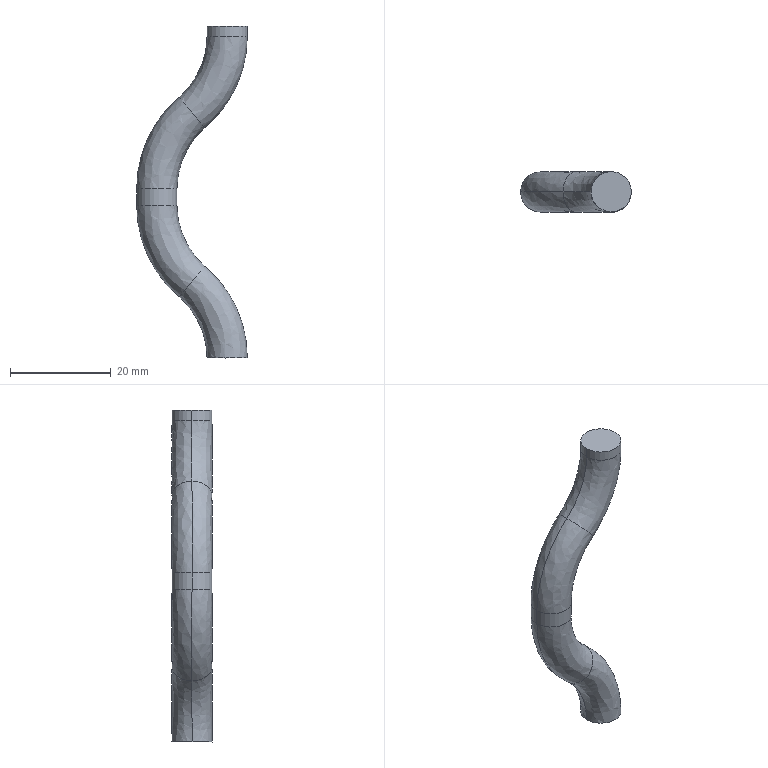Part | SolidWorks | features BaseBody 1 | 1 solid | 14 faces | box 22 x 8 x 66 mm | volume 3733 mm3 | spline 8 | cylinder 4 | plane 2 | commonest cylinder face diameters 8 x4
STEP:
#1=CARTESIAN_POINT('',(-10.,-0.000000001,280.603));
#2=VERTEX_POINT('',#1);
#3=CARTESIAN_POINT('',(-18.,0.,280.603));
#4=VERTEX_POINT('',#3);
#5=CARTESIAN_POINT('',(-14.,-0.000000001,280.603));
#6=DIRECTION('',(0.,0.,1.));
#7=DIRECTION('',(-1.,0.,0.));
#8=AXIS2_PLACEMENT_3D('',#5,#6,#7);
#9=CIRCLE('',#8,4.);
#10=EDGE_CURVE('',#2,#4,#9,.T.);
#11=ORIENTED_EDGE('',*,*,#10,.F.);
#12=CARTESIAN_POINT('',(-10.,-0.000000001,277.397));
#13=VERTEX_POINT('',#12);
#14=CARTESIAN_POINT('',(-10.,0.,280.603));
#15=DIRECTION('',(0.,0.,-1.));
#16=VECTOR('',#15,1000.);
#17=LINE('',#14,#16);
#18=EDGE_CURVE('',#2,#13,#17,.T.);
#19=ORIENTED_EDGE('',*,*,#18,.T.);
#20=CARTESIAN_POINT('',(-18.,0.,277.397));
#21=VERTEX_POINT('',#20);
#22=CARTESIAN_POINT('',(-14.,0.,277.397));
#23=DIRECTION('',(0.,0.,1.));
#24=DIRECTION('',(-1.,0.,0.));
#25=AXIS2_PLACEMENT_3D('',#22,#23,#24);
#26=CIRCLE('',#25,4.);
#27=EDGE_CURVE('',#13,#21,#26,.T.);
#28=ORIENTED_EDGE('',*,*,#27,.T.);
#29=CARTESIAN_POINT('',(-18.,0.,280.603));
#30=DIRECTION('',(0.,0.,-1.));
#31=VECTOR('',#30,1000.);
#32=LINE('',#29,#31);
#33=EDGE_CURVE('',#4,#21,#32,.T.);
#34=ORIENTED_EDGE('',*,*,#33,.F.);
#35=EDGE_LOOP('',(#11,#19,#28,#34));
#36=FACE_OUTER_BOUND('',#35,.T.);
#37=CARTESIAN_POINT('',(-14.,0.,280.603));
#38=DIRECTION('',(0.,0.,-1.));
#39=DIRECTION('',(-1.,0.,0.));
#40=AXIS2_PLACEMENT_3D('',#37,#38,#39);
#41=CYLINDRICAL_SURFACE('',#40,4.);
#42=ADVANCED_FACE('',(#36),#41,.T.);
#43=CARTESIAN_POINT('',(-4.,0.000000001,311.));
#44=VERTEX_POINT('',#43);
#45=CARTESIAN_POINT('',(4.,0.,311.));
#46=VERTEX_POINT('',#45);
#47=CARTESIAN_POINT('',(0.,0.,311.));
#48=DIRECTION('',(0.,0.,-1.));
#49=DIRECTION('',(1.,0.,0.));
#50=AXIS2_PLACEMENT_3D('',#47,#48,#49);
#51=CIRCLE('',#50,4.);
#52=EDGE_CURVE('',#44,#46,#51,.T.);
#53=ORIENTED_EDGE('',*,*,#52,.F.);
#54=CARTESIAN_POINT('',(-4.,0.,313.));
#55=VERTEX_POINT('',#54);
#56=CARTESIAN_POINT('',(-4.,0.,311.));
#57=DIRECTION('',(0.,0.,1.));
#58=VECTOR('',#57,1000.);
#59=LINE('',#56,#58);
#60=EDGE_CURVE('',#44,#55,#59,.T.);
#61=ORIENTED_EDGE('',*,*,#60,.T.);
#62=CARTESIAN_POINT('',(4.,0.,313.));
#63=VERTEX_POINT('',#62);
#64=CARTESIAN_POINT('',(0.,0.,313.));
#65=DIRECTION('',(0.,0.,-1.));
#66=DIRECTION('',(1.,0.,0.));
#67=AXIS2_PLACEMENT_3D('',#64,#65,#66);
#68=CIRCLE('',#67,4.);
#69=EDGE_CURVE('',#55,#63,#68,.T.);
#70=ORIENTED_EDGE('',*,*,#69,.T.);
#71=CARTESIAN_POINT('',(4.,0.,311.));
#72=DIRECTION('',(0.,0.,1.));
#73=VECTOR('',#72,1000.);
#74=LINE('',#71,#73);
#75=EDGE_CURVE('',#46,#63,#74,.T.);
#76=ORIENTED_EDGE('',*,*,#75,.F.);
#77=EDGE_LOOP('',(#53,#61,#70,#76));
#78=FACE_OUTER_BOUND('',#77,.T.);
#79=CARTESIAN_POINT('',(0.,0.,311.));
#80=DIRECTION('',(0.,0.,1.));
#81=DIRECTION('',(1.,0.,0.));
#82=AXIS2_PLACEMENT_3D('',#79,#80,#81);
#83=CYLINDRICAL_SURFACE('',#82,4.);
#84=ADVANCED_FACE('',(#78),#83,.T.);
#85=ORIENTED_EDGE('',*,*,#10,.T.);
#86=CARTESIAN_POINT('',(-9.6,0.000000001,298.841));
#87=VERTEX_POINT('',#86);
#88=CARTESIAN_POINT('',(6.,0.000000004,280.603));
#89=DIRECTION('',(0.,1.,0.));
#90=DIRECTION('',(-0.65,0.,0.7599));
#91=AXIS2_PLACEMENT_3D('',#88,#89,#90);
#92=CIRCLE('',#91,24.);
#93=EDGE_CURVE('',#4,#87,#92,.T.);
#94=ORIENTED_EDGE('',*,*,#93,.T.);
#95=CARTESIAN_POINT('',(-4.4,0.,292.762));
#96=VERTEX_POINT('',#95);
#97=CARTESIAN_POINT('',(-7.,0.000000001,295.801));
#98=DIRECTION('',(-0.7599,0.,-0.65));
#99=DIRECTION('',(-0.65,0.,0.7599));
#100=AXIS2_PLACEMENT_3D('',#97,#98,#99);
#101=CIRCLE('',#100,4.);
#102=EDGE_CURVE('',#87,#96,#101,.T.);
#103=ORIENTED_EDGE('',*,*,#102,.T.);
#104=CARTESIAN_POINT('',(6.,0.000000002,280.603));
#105=DIRECTION('',(0.,-1.,0.));
#106=DIRECTION('',(-0.65,0.,0.7599));
#107=AXIS2_PLACEMENT_3D('',#104,#105,#106);
#108=CIRCLE('',#107,16.);
#109=EDGE_CURVE('',#96,#2,#108,.T.);
#110=ORIENTED_EDGE('',*,*,#109,.T.);
#111=EDGE_LOOP('',(#85,#94,#103,#110));
#112=FACE_OUTER_BOUND('',#111,.T.);
#113=CARTESIAN_POINT('',(-9.6,0.000000001,298.841));
#114=CARTESIAN_POINT('',(-15.018,0.,294.207));
#115=CARTESIAN_POINT('',(-18.,-0.000000001,287.732));
#116=CARTESIAN_POINT('',(-18.,-0.000000001,280.603));
#117=CARTESIAN_POINT('',(-9.6,2.343,298.841));
#118=CARTESIAN_POINT('',(-15.018,2.343,294.207));
#119=CARTESIAN_POINT('',(-18.,2.343,287.732));
#120=CARTESIAN_POINT('',(-18.,2.343,280.603));
#121=CARTESIAN_POINT('',(-8.523,4.,297.582));
#122=CARTESIAN_POINT('',(-13.567,4.,293.268));
#123=CARTESIAN_POINT('',(-16.343,4.,287.24));
#124=CARTESIAN_POINT('',(-16.343,4.,280.603));
#125=CARTESIAN_POINT('',(-7.,4.,295.801));
#126=CARTESIAN_POINT('',(-11.515,4.,291.94));
#127=CARTESIAN_POINT('',(-14.,4.,286.544));
#128=CARTESIAN_POINT('',(-14.,4.,280.603));
#129=CARTESIAN_POINT('',(-5.477,4.,294.021));
#130=CARTESIAN_POINT('',(-9.463,4.,290.611));
#131=CARTESIAN_POINT('',(-11.657,4.,285.848));
#132=CARTESIAN_POINT('',(-11.657,4.,280.603));
#133=CARTESIAN_POINT('',(-4.4,2.343,292.762));
#134=CARTESIAN_POINT('',(-8.012,2.343,289.672));
#135=CARTESIAN_POINT('',(-10.,2.343,285.355));
#136=CARTESIAN_POINT('',(-10.,2.343,280.603));
#137=CARTESIAN_POINT('',(-4.4,0.,292.762));
#138=CARTESIAN_POINT('',(-8.012,-0.000000001,289.672));
#139=CARTESIAN_POINT('',(-10.,-0.000000002,285.355));
#140=CARTESIAN_POINT('',(-10.,-0.000000002,280.603));
#141=(BOUNDED_SURFACE()B_SPLINE_SURFACE(3,3,((#113,#114,#115,#116),(#117,#118,#119,#120),(#121,#122,#123,#124),(#125,#126,#127,#128),(#129,#130,#131,#132),(#133,#134,#135,#136),(#137,#138,#139,#140)),.UNSPECIFIED.,.F.,.F.,.T.)B_SPLINE_SURFACE_WITH_KNOTS((4,3,4),(4,4),(0.,0.5,1.),(0.,1.),.UNSPECIFIED.)GEOMETRIC_REPRESENTATION_ITEM()RATIONAL_B_SPLINE_SURFACE(((1.,0.9389,0.9389,1.),(0.8047,0.7555,0.7555,0.8047),(0.8047,0.7555,0.7555,0.8047),(1.,0.9389,0.9389,1.),(0.8047,0.7555,0.7555,0.8047),(0.8047,0.7555,0.7555,0.8047),(1.,0.9389,0.9389,1.)))REPRESENTATION_ITEM('')SURFACE());
#142=ADVANCED_FACE('',(#112),#141,.T.);
#143=ORIENTED_EDGE('',*,*,#109,.F.);
#144=CARTESIAN_POINT('',(-7.,-0.000000001,295.801));
#145=DIRECTION('',(-0.7599,0.,-0.65));
#146=DIRECTION('',(-0.65,0.,0.7599));
#147=AXIS2_PLACEMENT_3D('',#144,#145,#146);
#148=CIRCLE('',#147,4.);
#149=EDGE_CURVE('',#96,#87,#148,.T.);
#150=ORIENTED_EDGE('',*,*,#149,.T.);
#151=ORIENTED_EDGE('',*,*,#93,.F.);
#152=CARTESIAN_POINT('',(-14.,0.000000001,280.603));
#153=DIRECTION('',(0.,0.,1.));
#154=DIRECTION('',(-1.,0.,0.));
#155=AXIS2_PLACEMENT_3D('',#152,#153,#154);
#156=CIRCLE('',#155,4.);
#157=EDGE_CURVE('',#4,#2,#156,.T.);
#158=ORIENTED_EDGE('',*,*,#157,.T.);
#159=EDGE_LOOP('',(#143,#150,#151,#158));
#160=FACE_OUTER_BOUND('',#159,.T.);
#161=CARTESIAN_POINT('',(-18.,0.000000003,280.603));
#162=CARTESIAN_POINT('',(-18.,0.000000003,287.732));
#163=CARTESIAN_POINT('',(-15.018,0.000000002,294.207));
#164=CARTESIAN_POINT('',(-9.6,0.000000001,298.841));
#165=CARTESIAN_POINT('',(-18.,-2.343,280.603));
#166=CARTESIAN_POINT('',(-18.,-2.343,287.732));
#167=CARTESIAN_POINT('',(-15.018,-2.343,294.207));
#168=CARTESIAN_POINT('',(-9.6,-2.343,298.841));
#169=CARTESIAN_POINT('',(-16.343,-4.,280.603));
#170=CARTESIAN_POINT('',(-16.343,-4.,287.24));
#171=CARTESIAN_POINT('',(-13.567,-4.,293.268));
#172=CARTESIAN_POINT('',(-8.523,-4.,297.582));
#173=CARTESIAN_POINT('',(-14.,-4.,280.603));
#174=CARTESIAN_POINT('',(-14.,-4.,286.544));
#175=CARTESIAN_POINT('',(-11.515,-4.,291.94));
#176=CARTESIAN_POINT('',(-7.,-4.,295.801));
#177=CARTESIAN_POINT('',(-11.657,-4.,280.603));
#178=CARTESIAN_POINT('',(-11.657,-4.,285.848));
#179=CARTESIAN_POINT('',(-9.463,-4.,290.611));
#180=CARTESIAN_POINT('',(-5.477,-4.,294.021));
#181=CARTESIAN_POINT('',(-10.,-2.343,280.603));
#182=CARTESIAN_POINT('',(-10.,-2.343,285.355));
#183=CARTESIAN_POINT('',(-8.012,-2.343,289.672));
#184=CARTESIAN_POINT('',(-4.4,-2.343,292.762));
#185=CARTESIAN_POINT('',(-10.,0.000000001,280.603));
#186=CARTESIAN_POINT('',(-10.,0.000000001,285.355));
#187=CARTESIAN_POINT('',(-8.012,0.000000001,289.672));
#188=CARTESIAN_POINT('',(-4.4,0.,292.762));
#189=(BOUNDED_SURFACE()B_SPLINE_SURFACE(3,3,((#161,#162,#163,#164),(#165,#166,#167,#168),(#169,#170,#171,#172),(#173,#174,#175,#176),(#177,#178,#179,#180),(#181,#182,#183,#184),(#185,#186,#187,#188)),.UNSPECIFIED.,.F.,.F.,.T.)B_SPLINE_SURFACE_WITH_KNOTS((4,3,4),(4,4),(0.,0.5,1.),(0.,1.),.UNSPECIFIED.)GEOMETRIC_REPRESENTATION_ITEM()RATIONAL_B_SPLINE_SURFACE(((1.,0.9389,0.9389,1.),(0.8047,0.7555,0.7555,0.8047),(0.8047,0.7555,0.7555,0.8047),(1.,0.9389,0.9389,1.),(0.8047,0.7555,0.7555,0.8047),(0.8047,0.7555,0.7555,0.8047),(1.,0.9389,0.9389,1.)))REPRESENTATION_ITEM('')SURFACE());
#190=ADVANCED_FACE('',(#160),#189,.T.);
#191=ORIENTED_EDGE('',*,*,#18,.F.);
#192=ORIENTED_EDGE('',*,*,#157,.F.);
#193=ORIENTED_EDGE('',*,*,#33,.T.);
#194=CARTESIAN_POINT('',(-14.,0.,277.397));
#195=DIRECTION('',(0.,0.,1.));
#196=DIRECTION('',(-1.,0.,0.));
#197=AXIS2_PLACEMENT_3D('',#194,#195,#196);
#198=CIRCLE('',#197,4.);
#199=EDGE_CURVE('',#21,#13,#198,.T.);
#200=ORIENTED_EDGE('',*,*,#199,.T.);
#201=EDGE_LOOP('',(#191,#192,#193,#200));
#202=FACE_OUTER_BOUND('',#201,.T.);
#203=CARTESIAN_POINT('',(-14.,0.,280.603));
#204=DIRECTION('',(0.,0.,-1.));
#205=DIRECTION('',(-1.,0.,0.));
#206=AXIS2_PLACEMENT_3D('',#203,#204,#205);
#207=CYLINDRICAL_SURFACE('',#206,4.);
#208=ADVANCED_FACE('',(#202),#207,.T.);
#209=CARTESIAN_POINT('',(-20.,-0.000000002,311.));
#210=DIRECTION('',(0.,-1.,0.));
#211=DIRECTION('',(1.,0.,0.));
#212=AXIS2_PLACEMENT_3D('',#209,#210,#211);
#213=CIRCLE('',#212,16.);
#214=EDGE_CURVE('',#87,#44,#213,.T.);
#215=ORIENTED_EDGE('',*,*,#214,.T.);
#216=ORIENTED_EDGE('',*,*,#52,.T.);
#217=CARTESIAN_POINT('',(-20.,-0.000000004,311.));
#218=DIRECTION('',(0.,1.,0.));
#219=DIRECTION('',(1.,0.,0.));
#220=AXIS2_PLACEMENT_3D('',#217,#218,#219);
#221=CIRCLE('',#220,24.);
#222=EDGE_CURVE('',#46,#96,#221,.T.);
#223=ORIENTED_EDGE('',*,*,#222,.T.);
#224=ORIENTED_EDGE('',*,*,#102,.F.);
#225=EDGE_LOOP('',(#215,#216,#223,#224));
#226=FACE_OUTER_BOUND('',#225,.T.);
#227=CARTESIAN_POINT('',(-4.4,0.,292.762));
#228=CARTESIAN_POINT('',(1.018,0.,297.396));
#229=CARTESIAN_POINT('',(4.,0.,303.871));
#230=CARTESIAN_POINT('',(4.,0.,311.));
#231=CARTESIAN_POINT('',(-4.4,8.,292.762));
#232=CARTESIAN_POINT('',(1.018,8.,297.396));
#233=CARTESIAN_POINT('',(4.,8.,303.871));
#234=CARTESIAN_POINT('',(4.,8.,311.));
#235=CARTESIAN_POINT('',(-9.6,8.,298.841));
#236=CARTESIAN_POINT('',(-5.988,8.,301.93));
#237=CARTESIAN_POINT('',(-4.,8.,306.247));
#238=CARTESIAN_POINT('',(-4.,8.,311.));
#239=CARTESIAN_POINT('',(-9.6,0.000000001,298.841));
#240=CARTESIAN_POINT('',(-5.988,0.000000001,301.93));
#241=CARTESIAN_POINT('',(-4.,0.000000001,306.247));
#242=CARTESIAN_POINT('',(-4.,0.000000001,311.));
#243=(BOUNDED_SURFACE()B_SPLINE_SURFACE(3,3,((#227,#228,#229,#230),(#231,#232,#233,#234),(#235,#236,#237,#238),(#239,#240,#241,#242)),.UNSPECIFIED.,.F.,.F.,.T.)B_SPLINE_SURFACE_WITH_KNOTS((4,4),(4,4),(0.,1.),(0.,1.),.UNSPECIFIED.)GEOMETRIC_REPRESENTATION_ITEM()RATIONAL_B_SPLINE_SURFACE(((1.,0.9389,0.9389,1.),(0.3333,0.313,0.313,0.3333),(0.3333,0.313,0.313,0.3333),(1.,0.9389,0.9389,1.)))REPRESENTATION_ITEM('')SURFACE());
#244=ADVANCED_FACE('',(#226),#243,.T.);
#245=ORIENTED_EDGE('',*,*,#222,.F.);
#246=CARTESIAN_POINT('',(0.,0.,311.));
#247=DIRECTION('',(0.,0.,-1.));
#248=DIRECTION('',(1.,0.,0.));
#249=AXIS2_PLACEMENT_3D('',#246,#247,#248);
#250=CIRCLE('',#249,4.);
#251=EDGE_CURVE('',#46,#44,#250,.T.);
#252=ORIENTED_EDGE('',*,*,#251,.T.);
#253=ORIENTED_EDGE('',*,*,#214,.F.);
#254=ORIENTED_EDGE('',*,*,#149,.F.);
#255=EDGE_LOOP('',(#245,#252,#253,#254));
#256=FACE_OUTER_BOUND('',#255,.T.);
#257=CARTESIAN_POINT('',(4.,0.000000001,311.));
#258=CARTESIAN_POINT('',(4.,0.,303.871));
#259=CARTESIAN_POINT('',(1.018,0.,297.396));
#260=CARTESIAN_POINT('',(-4.4,0.000000001,292.762));
#261=CARTESIAN_POINT('',(4.,-2.343,311.));
#262=CARTESIAN_POINT('',(4.,-2.343,303.871));
#263=CARTESIAN_POINT('',(1.018,-2.343,297.396));
#264=CARTESIAN_POINT('',(-4.4,-2.343,292.762));
#265=CARTESIAN_POINT('',(2.343,-4.,311.));
#266=CARTESIAN_POINT('',(2.343,-4.,304.363));
#267=CARTESIAN_POINT('',(-0.4333,-4.,298.335));
#268=CARTESIAN_POINT('',(-5.477,-4.,294.021));
#269=CARTESIAN_POINT('',(0.,-4.,311.));
#270=CARTESIAN_POINT('',(0.,-4.,305.059));
#271=CARTESIAN_POINT('',(-2.485,-4.,299.663));
#272=CARTESIAN_POINT('',(-7.,-4.,295.801));
#273=CARTESIAN_POINT('',(-2.343,-4.,311.));
#274=CARTESIAN_POINT('',(-2.343,-4.,305.755));
#275=CARTESIAN_POINT('',(-4.537,-4.,300.991));
#276=CARTESIAN_POINT('',(-8.523,-4.,297.582));
#277=CARTESIAN_POINT('',(-4.,-2.343,311.));
#278=CARTESIAN_POINT('',(-4.,-2.343,306.247));
#279=CARTESIAN_POINT('',(-5.988,-2.343,301.93));
#280=CARTESIAN_POINT('',(-9.6,-2.343,298.841));
#281=CARTESIAN_POINT('',(-4.,0.000000001,311.));
#282=CARTESIAN_POINT('',(-4.,0.000000001,306.247));
#283=CARTESIAN_POINT('',(-5.988,0.000000001,301.93));
#284=CARTESIAN_POINT('',(-9.6,0.000000001,298.841));
#285=(BOUNDED_SURFACE()B_SPLINE_SURFACE(3,3,((#257,#258,#259,#260),(#261,#262,#263,#264),(#265,#266,#267,#268),(#269,#270,#271,#272),(#273,#274,#275,#276),(#277,#278,#279,#280),(#281,#282,#283,#284)),.UNSPECIFIED.,.F.,.F.,.T.)B_SPLINE_SURFACE_WITH_KNOTS((4,3,4),(4,4),(0.,0.5,1.),(0.,1.),.UNSPECIFIED.)GEOMETRIC_REPRESENTATION_ITEM()RATIONAL_B_SPLINE_SURFACE(((1.,0.9389,0.9389,1.),(0.8047,0.7555,0.7555,0.8047),(0.8047,0.7555,0.7555,0.8047),(1.,0.9389,0.9389,1.),(0.8047,0.7555,0.7555,0.8047),(0.8047,0.7555,0.7555,0.8047),(1.,0.9389,0.9389,1.)))REPRESENTATION_ITEM('')SURFACE());
#286=ADVANCED_FACE('',(#256),#285,.T.);
#287=CARTESIAN_POINT('',(-4.4,0.,265.238));
#288=VERTEX_POINT('',#287);
#289=CARTESIAN_POINT('',(-9.6,0.000000001,259.159));
#290=VERTEX_POINT('',#289);
#291=CARTESIAN_POINT('',(-7.,0.,262.199));
#292=DIRECTION('',(-0.7599,0.,0.65));
#293=DIRECTION('',(-0.65,0.,-0.7599));
#294=AXIS2_PLACEMENT_3D('',#291,#292,#293);
#295=CIRCLE('',#294,4.);
#296=EDGE_CURVE('',#288,#290,#295,.T.);
#297=ORIENTED_EDGE('',*,*,#296,.T.);
#298=CARTESIAN_POINT('',(6.,-0.000000004,277.397));
#299=DIRECTION('',(0.,1.,0.));
#300=DIRECTION('',(-1.,0.,0.));
#301=AXIS2_PLACEMENT_3D('',#298,#299,#300);
#302=CIRCLE('',#301,24.);
#303=EDGE_CURVE('',#290,#21,#302,.T.);
#304=ORIENTED_EDGE('',*,*,#303,.T.);
#305=ORIENTED_EDGE('',*,*,#27,.F.);
#306=CARTESIAN_POINT('',(6.,-0.000000005,277.397));
#307=DIRECTION('',(0.,-1.,0.));
#308=DIRECTION('',(-1.,0.,0.));
#309=AXIS2_PLACEMENT_3D('',#306,#307,#308);
#310=CIRCLE('',#309,16.);
#311=EDGE_CURVE('',#13,#288,#310,.T.);
#312=ORIENTED_EDGE('',*,*,#311,.T.);
#313=EDGE_LOOP('',(#297,#304,#305,#312));
#314=FACE_OUTER_BOUND('',#313,.T.);
#315=CARTESIAN_POINT('',(-18.,0.,277.397));
#316=CARTESIAN_POINT('',(-18.,0.000000001,270.268));
#317=CARTESIAN_POINT('',(-15.018,0.000000001,263.793));
#318=CARTESIAN_POINT('',(-9.6,0.,259.159));
#319=CARTESIAN_POINT('',(-18.,2.343,277.397));
#320=CARTESIAN_POINT('',(-18.,2.343,270.268));
#321=CARTESIAN_POINT('',(-15.018,2.343,263.793));
#322=CARTESIAN_POINT('',(-9.6,2.343,259.159));
#323=CARTESIAN_POINT('',(-16.343,4.,277.397));
#324=CARTESIAN_POINT('',(-16.343,4.,270.76));
#325=CARTESIAN_POINT('',(-13.567,4.,264.732));
#326=CARTESIAN_POINT('',(-8.523,4.,260.418));
#327=CARTESIAN_POINT('',(-14.,4.,277.397));
#328=CARTESIAN_POINT('',(-14.,4.,271.456));
#329=CARTESIAN_POINT('',(-11.515,4.,266.06));
#330=CARTESIAN_POINT('',(-7.,4.,262.199));
#331=CARTESIAN_POINT('',(-11.657,4.,277.397));
#332=CARTESIAN_POINT('',(-11.657,4.,272.152));
#333=CARTESIAN_POINT('',(-9.463,4.,267.389));
#334=CARTESIAN_POINT('',(-5.477,4.,263.979));
#335=CARTESIAN_POINT('',(-10.,2.343,277.397));
#336=CARTESIAN_POINT('',(-10.,2.343,272.645));
#337=CARTESIAN_POINT('',(-8.012,2.343,268.328));
#338=CARTESIAN_POINT('',(-4.4,2.343,265.238));
#339=CARTESIAN_POINT('',(-10.,-0.000000002,277.397));
#340=CARTESIAN_POINT('',(-10.,-0.000000001,272.645));
#341=CARTESIAN_POINT('',(-8.012,-0.000000001,268.328));
#342=CARTESIAN_POINT('',(-4.4,-0.000000002,265.238));
#343=(BOUNDED_SURFACE()B_SPLINE_SURFACE(3,3,((#315,#316,#317,#318),(#319,#320,#321,#322),(#323,#324,#325,#326),(#327,#328,#329,#330),(#331,#332,#333,#334),(#335,#336,#337,#338),(#339,#340,#341,#342)),.UNSPECIFIED.,.F.,.F.,.T.)B_SPLINE_SURFACE_WITH_KNOTS((4,3,4),(4,4),(0.,0.5,1.),(0.,1.),.UNSPECIFIED.)GEOMETRIC_REPRESENTATION_ITEM()RATIONAL_B_SPLINE_SURFACE(((1.,0.9389,0.9389,1.),(0.8047,0.7555,0.7555,0.8047),(0.8047,0.7555,0.7555,0.8047),(1.,0.9389,0.9389,1.),(0.8047,0.7555,0.7555,0.8047),(0.8047,0.7555,0.7555,0.8047),(1.,0.9389,0.9389,1.)))REPRESENTATION_ITEM('')SURFACE());
#344=ADVANCED_FACE('',(#314),#343,.T.);
#345=ORIENTED_EDGE('',*,*,#60,.F.);
#346=ORIENTED_EDGE('',*,*,#251,.F.);
#347=ORIENTED_EDGE('',*,*,#75,.T.);
#348=CARTESIAN_POINT('',(0.,0.,313.));
#349=DIRECTION('',(0.,0.,-1.));
#350=DIRECTION('',(1.,0.,0.));
#351=AXIS2_PLACEMENT_3D('',#348,#349,#350);
#352=CIRCLE('',#351,4.);
#353=EDGE_CURVE('',#63,#55,#352,.T.);
#354=ORIENTED_EDGE('',*,*,#353,.T.);
#355=EDGE_LOOP('',(#345,#346,#347,#354));
#356=FACE_OUTER_BOUND('',#355,.T.);
#357=CARTESIAN_POINT('',(0.,0.,311.));
#358=DIRECTION('',(0.,0.,1.));
#359=DIRECTION('',(1.,0.,0.));
#360=AXIS2_PLACEMENT_3D('',#357,#358,#359);
#361=CYLINDRICAL_SURFACE('',#360,4.);
#362=ADVANCED_FACE('',(#356),#361,.T.);
#363=ORIENTED_EDGE('',*,*,#311,.F.);
#364=ORIENTED_EDGE('',*,*,#199,.F.);
#365=ORIENTED_EDGE('',*,*,#303,.F.);
#366=CARTESIAN_POINT('',(-7.,0.,262.199));
#367=DIRECTION('',(-0.7599,0.,0.65));
#368=DIRECTION('',(-0.65,0.,-0.7599));
#369=AXIS2_PLACEMENT_3D('',#366,#367,#368);
#370=CIRCLE('',#369,4.);
#371=EDGE_CURVE('',#290,#288,#370,.T.);
#372=ORIENTED_EDGE('',*,*,#371,.T.);
#373=EDGE_LOOP('',(#363,#364,#365,#372));
#374=FACE_OUTER_BOUND('',#373,.T.);
#375=CARTESIAN_POINT('',(-9.6,0.000000001,259.159));
#376=CARTESIAN_POINT('',(-15.018,0.,263.793));
#377=CARTESIAN_POINT('',(-18.,0.,270.268));
#378=CARTESIAN_POINT('',(-18.,0.000000001,277.397));
#379=CARTESIAN_POINT('',(-9.6,-2.343,259.159));
#380=CARTESIAN_POINT('',(-15.018,-2.343,263.793));
#381=CARTESIAN_POINT('',(-18.,-2.343,270.268));
#382=CARTESIAN_POINT('',(-18.,-2.343,277.397));
#383=CARTESIAN_POINT('',(-8.523,-4.,260.418));
#384=CARTESIAN_POINT('',(-13.567,-4.,264.732));
#385=CARTESIAN_POINT('',(-16.343,-4.,270.76));
#386=CARTESIAN_POINT('',(-16.343,-4.,277.397));
#387=CARTESIAN_POINT('',(-7.,-4.,262.199));
#388=CARTESIAN_POINT('',(-11.515,-4.,266.06));
#389=CARTESIAN_POINT('',(-14.,-4.,271.456));
#390=CARTESIAN_POINT('',(-14.,-4.,277.397));
#391=CARTESIAN_POINT('',(-5.477,-4.,263.979));
#392=CARTESIAN_POINT('',(-9.463,-4.,267.389));
#393=CARTESIAN_POINT('',(-11.657,-4.,272.152));
#394=CARTESIAN_POINT('',(-11.657,-4.,277.397));
#395=CARTESIAN_POINT('',(-4.4,-2.343,265.238));
#396=CARTESIAN_POINT('',(-8.012,-2.343,268.328));
#397=CARTESIAN_POINT('',(-10.,-2.343,272.645));
#398=CARTESIAN_POINT('',(-10.,-2.343,277.397));
#399=CARTESIAN_POINT('',(-4.4,0.,265.238));
#400=CARTESIAN_POINT('',(-8.012,0.,268.328));
#401=CARTESIAN_POINT('',(-10.,0.,272.645));
#402=CARTESIAN_POINT('',(-10.,0.,277.397));
#403=(BOUNDED_SURFACE()B_SPLINE_SURFACE(3,3,((#375,#376,#377,#378),(#379,#380,#381,#382),(#383,#384,#385,#386),(#387,#388,#389,#390),(#391,#392,#393,#394),(#395,#396,#397,#398),(#399,#400,#401,#402)),.UNSPECIFIED.,.F.,.F.,.T.)B_SPLINE_SURFACE_WITH_KNOTS((4,3,4),(4,4),(0.,0.5,1.),(0.,1.),.UNSPECIFIED.)GEOMETRIC_REPRESENTATION_ITEM()RATIONAL_B_SPLINE_SURFACE(((1.,0.9389,0.9389,1.),(0.8047,0.7555,0.7555,0.8047),(0.8047,0.7555,0.7555,0.8047),(1.,0.9389,0.9389,1.),(0.8047,0.7555,0.7555,0.8047),(0.8047,0.7555,0.7555,0.8047),(1.,0.9389,0.9389,1.)))REPRESENTATION_ITEM('')SURFACE());
#404=ADVANCED_FACE('',(#374),#403,.T.);
#405=CARTESIAN_POINT('',(-4.,0.,247.));
#406=VERTEX_POINT('',#405);
#407=CARTESIAN_POINT('',(-20.,0.000000004,247.));
#408=DIRECTION('',(0.,-1.,0.));
#409=DIRECTION('',(0.65,0.,0.7599));
#410=AXIS2_PLACEMENT_3D('',#407,#408,#409);
#411=CIRCLE('',#410,16.);
#412=EDGE_CURVE('',#406,#290,#411,.T.);
#413=ORIENTED_EDGE('',*,*,#412,.T.);
#414=ORIENTED_EDGE('',*,*,#296,.F.);
#415=CARTESIAN_POINT('',(4.,0.,247.));
#416=VERTEX_POINT('',#415);
#417=CARTESIAN_POINT('',(-20.,0.000000004,247.));
#418=DIRECTION('',(0.,1.,0.));
#419=DIRECTION('',(0.65,0.,0.7599));
#420=AXIS2_PLACEMENT_3D('',#417,#418,#419);
#421=CIRCLE('',#420,24.);
#422=EDGE_CURVE('',#288,#416,#421,.T.);
#423=ORIENTED_EDGE('',*,*,#422,.T.);
#424=CARTESIAN_POINT('',(4.,0.,247.));
#425=CARTESIAN_POINT('',(4.,0.2642,247.));
#426=CARTESIAN_POINT('',(3.974,0.5241,247.));
#427=CARTESIAN_POINT('',(3.872,1.035,247.));
#428=CARTESIAN_POINT('',(3.796,1.289,247.));
#429=CARTESIAN_POINT('',(3.595,1.774,247.));
#430=CARTESIAN_POINT('',(3.472,2.003,247.));
#431=CARTESIAN_POINT('',(3.182,2.438,247.));
#432=CARTESIAN_POINT('',(3.013,2.644,247.));
#433=CARTESIAN_POINT('',(2.644,3.013,247.));
#434=CARTESIAN_POINT('',(2.443,3.179,247.));
#435=CARTESIAN_POINT('',(2.005,3.471,247.));
#436=CARTESIAN_POINT('',(1.773,3.595,247.));
#437=CARTESIAN_POINT('',(1.291,3.795,247.));
#438=CARTESIAN_POINT('',(1.039,3.872,247.));
#439=CARTESIAN_POINT('',(0.523,3.974,247.));
#440=CARTESIAN_POINT('',(0.2635,4.,247.));
#441=CARTESIAN_POINT('',(-0.2581,4.,247.));
#442=CARTESIAN_POINT('',(-0.5231,3.974,247.));
#443=CARTESIAN_POINT('',(-1.036,3.872,247.));
#444=CARTESIAN_POINT('',(-1.285,3.797,247.));
#445=CARTESIAN_POINT('',(-1.77,3.597,247.));
#446=CARTESIAN_POINT('',(-2.004,3.472,247.));
#447=CARTESIAN_POINT('',(-2.437,3.182,247.));
#448=CARTESIAN_POINT('',(-2.64,3.017,247.));
#449=CARTESIAN_POINT('',(-3.013,2.644,247.));
#450=CARTESIAN_POINT('',(-3.179,2.442,247.));
#451=CARTESIAN_POINT('',(-3.469,2.009,247.));
#452=CARTESIAN_POINT('',(-3.594,1.775,247.));
#453=CARTESIAN_POINT('',(-3.795,1.29,247.));
#454=CARTESIAN_POINT('',(-3.871,1.041,247.));
#455=CARTESIAN_POINT('',(-3.974,0.5286,247.));
#456=CARTESIAN_POINT('',(-4.,0.2642,247.));
#457=CARTESIAN_POINT('',(-4.,0.,247.));
#458=B_SPLINE_CURVE_WITH_KNOTS('',3,(#424,#425,#426,#427,#428,#429,#430,#431,#432,#433,#434,#435,#436,#437,#438,#439,#440,#441,#442,#443,#444,#445,#446,#447,#448,#449,#450,#451,#452,#453,#454,#455,#456,#457),.UNSPECIFIED.,.F.,.F.,(4,2,2,2,2,2,2,2,2,2,2,2,2,2,2,2,4),(0.,0.0007815,0.001563,0.002344,0.003126,0.003907,0.004689,0.00547,0.006252,0.007033,0.007815,0.008596,0.009377,0.01016,0.01094,0.01172,0.0125),.UNSPECIFIED.);
#459=EDGE_CURVE('',#416,#406,#458,.T.);
#460=ORIENTED_EDGE('',*,*,#459,.T.);
#461=EDGE_LOOP('',(#413,#414,#423,#460));
#462=FACE_OUTER_BOUND('',#461,.T.);
#463=CARTESIAN_POINT('',(4.,-0.000000002,247.));
#464=CARTESIAN_POINT('',(4.,-0.000000002,254.129));
#465=CARTESIAN_POINT('',(1.018,-0.000000001,260.604));
#466=CARTESIAN_POINT('',(-4.4,0.,265.238));
#467=CARTESIAN_POINT('',(4.,2.343,247.));
#468=CARTESIAN_POINT('',(4.,2.343,254.129));
#469=CARTESIAN_POINT('',(1.018,2.343,260.604));
#470=CARTESIAN_POINT('',(-4.4,2.343,265.238));
#471=CARTESIAN_POINT('',(2.343,4.,247.));
#472=CARTESIAN_POINT('',(2.343,4.,253.637));
#473=CARTESIAN_POINT('',(-0.4333,4.,259.665));
#474=CARTESIAN_POINT('',(-5.477,4.,263.979));
#475=CARTESIAN_POINT('',(0.,4.,247.));
#476=CARTESIAN_POINT('',(0.,4.,252.941));
#477=CARTESIAN_POINT('',(-2.485,4.,258.337));
#478=CARTESIAN_POINT('',(-7.,4.,262.199));
#479=CARTESIAN_POINT('',(-2.343,4.,247.));
#480=CARTESIAN_POINT('',(-2.343,4.,252.245));
#481=CARTESIAN_POINT('',(-4.537,4.,257.009));
#482=CARTESIAN_POINT('',(-8.523,4.,260.418));
#483=CARTESIAN_POINT('',(-4.,2.343,247.));
#484=CARTESIAN_POINT('',(-4.,2.343,251.753));
#485=CARTESIAN_POINT('',(-5.988,2.343,256.07));
#486=CARTESIAN_POINT('',(-9.6,2.343,259.159));
#487=CARTESIAN_POINT('',(-4.,-0.000000001,247.));
#488=CARTESIAN_POINT('',(-4.,-0.000000001,251.753));
#489=CARTESIAN_POINT('',(-5.988,0.,256.07));
#490=CARTESIAN_POINT('',(-9.6,0.000000001,259.159));
#491=(BOUNDED_SURFACE()B_SPLINE_SURFACE(3,3,((#463,#464,#465,#466),(#467,#468,#469,#470),(#471,#472,#473,#474),(#475,#476,#477,#478),(#479,#480,#481,#482),(#483,#484,#485,#486),(#487,#488,#489,#490)),.UNSPECIFIED.,.F.,.F.,.T.)B_SPLINE_SURFACE_WITH_KNOTS((4,3,4),(4,4),(0.,0.5,1.),(0.,1.),.UNSPECIFIED.)GEOMETRIC_REPRESENTATION_ITEM()RATIONAL_B_SPLINE_SURFACE(((1.,0.9389,0.9389,1.),(0.8047,0.7555,0.7555,0.8047),(0.8047,0.7555,0.7555,0.8047),(1.,0.9389,0.9389,1.),(0.8047,0.7555,0.7555,0.8047),(0.8047,0.7555,0.7555,0.8047),(1.,0.9389,0.9389,1.)))REPRESENTATION_ITEM('')SURFACE());
#492=ADVANCED_FACE('',(#462),#491,.T.);
#493=ORIENTED_EDGE('',*,*,#353,.F.);
#494=ORIENTED_EDGE('',*,*,#69,.F.);
#495=EDGE_LOOP('',(#493,#494));
#496=FACE_OUTER_BOUND('',#495,.T.);
#497=CARTESIAN_POINT('',(0.,0.,313.));
#498=DIRECTION('',(0.,0.,1.));
#499=DIRECTION('',(1.,0.,0.));
#500=AXIS2_PLACEMENT_3D('',#497,#498,#499);
#501=PLANE('',#500);
#502=ADVANCED_FACE('',(#496),#501,.T.);
#503=CARTESIAN_POINT('',(-4.,0.,247.));
#504=CARTESIAN_POINT('',(-4.,-0.2642,247.));
#505=CARTESIAN_POINT('',(-3.974,-0.5241,247.));
#506=CARTESIAN_POINT('',(-3.872,-1.035,247.));
#507=CARTESIAN_POINT('',(-3.796,-1.289,247.));
#508=CARTESIAN_POINT('',(-3.595,-1.774,247.));
#509=CARTESIAN_POINT('',(-3.472,-2.003,247.));
#510=CARTESIAN_POINT('',(-3.182,-2.438,247.));
#511=CARTESIAN_POINT('',(-3.013,-2.644,247.));
#512=CARTESIAN_POINT('',(-2.644,-3.013,247.));
#513=CARTESIAN_POINT('',(-2.443,-3.179,247.));
#514=CARTESIAN_POINT('',(-2.005,-3.471,247.));
#515=CARTESIAN_POINT('',(-1.773,-3.595,247.));
#516=CARTESIAN_POINT('',(-1.291,-3.795,247.));
#517=CARTESIAN_POINT('',(-1.039,-3.872,247.));
#518=CARTESIAN_POINT('',(-0.523,-3.974,247.));
#519=CARTESIAN_POINT('',(-0.2635,-4.,247.));
#520=CARTESIAN_POINT('',(0.2581,-4.,247.));
#521=CARTESIAN_POINT('',(0.5231,-3.974,247.));
#522=CARTESIAN_POINT('',(1.036,-3.872,247.));
#523=CARTESIAN_POINT('',(1.285,-3.797,247.));
#524=CARTESIAN_POINT('',(1.77,-3.597,247.));
#525=CARTESIAN_POINT('',(2.004,-3.472,247.));
#526=CARTESIAN_POINT('',(2.437,-3.182,247.));
#527=CARTESIAN_POINT('',(2.64,-3.017,247.));
#528=CARTESIAN_POINT('',(3.013,-2.644,247.));
#529=CARTESIAN_POINT('',(3.179,-2.442,247.));
#530=CARTESIAN_POINT('',(3.469,-2.009,247.));
#531=CARTESIAN_POINT('',(3.594,-1.775,247.));
#532=CARTESIAN_POINT('',(3.795,-1.29,247.));
#533=CARTESIAN_POINT('',(3.871,-1.041,247.));
#534=CARTESIAN_POINT('',(3.974,-0.5286,247.));
#535=CARTESIAN_POINT('',(4.,-0.2642,247.));
#536=CARTESIAN_POINT('',(4.,0.,247.));
#537=B_SPLINE_CURVE_WITH_KNOTS('',3,(#503,#504,#505,#506,#507,#508,#509,#510,#511,#512,#513,#514,#515,#516,#517,#518,#519,#520,#521,#522,#523,#524,#525,#526,#527,#528,#529,#530,#531,#532,#533,#534,#535,#536),.UNSPECIFIED.,.F.,.F.,(4,2,2,2,2,2,2,2,2,2,2,2,2,2,2,2,4),(0.,0.0007815,0.001563,0.002344,0.003126,0.003907,0.004689,0.00547,0.006252,0.007033,0.007815,0.008596,0.009377,0.01016,0.01094,0.01172,0.0125),.UNSPECIFIED.);
#538=EDGE_CURVE('',#406,#416,#537,.T.);
#539=ORIENTED_EDGE('',*,*,#538,.T.);
#540=ORIENTED_EDGE('',*,*,#422,.F.);
#541=ORIENTED_EDGE('',*,*,#371,.F.);
#542=ORIENTED_EDGE('',*,*,#412,.F.);
#543=EDGE_LOOP('',(#539,#540,#541,#542));
#544=FACE_OUTER_BOUND('',#543,.T.);
#545=CARTESIAN_POINT('',(-4.4,0.,265.238));
#546=CARTESIAN_POINT('',(1.018,0.000000002,260.604));
#547=CARTESIAN_POINT('',(4.,0.000000002,254.129));
#548=CARTESIAN_POINT('',(4.,0.000000002,247.));
#549=CARTESIAN_POINT('',(-4.4,-2.343,265.238));
#550=CARTESIAN_POINT('',(1.018,-2.343,260.604));
#551=CARTESIAN_POINT('',(4.,-2.343,254.129));
#552=CARTESIAN_POINT('',(4.,-2.343,247.));
#553=CARTESIAN_POINT('',(-5.477,-4.,263.979));
#554=CARTESIAN_POINT('',(-0.4333,-4.,259.665));
#555=CARTESIAN_POINT('',(2.343,-4.,253.637));
#556=CARTESIAN_POINT('',(2.343,-4.,247.));
#557=CARTESIAN_POINT('',(-7.,-4.,262.199));
#558=CARTESIAN_POINT('',(-2.485,-4.,258.337));
#559=CARTESIAN_POINT('',(0.,-4.,252.941));
#560=CARTESIAN_POINT('',(0.,-4.,247.));
#561=CARTESIAN_POINT('',(-8.523,-4.,260.418));
#562=CARTESIAN_POINT('',(-4.537,-4.,257.009));
#563=CARTESIAN_POINT('',(-2.343,-4.,252.245));
#564=CARTESIAN_POINT('',(-2.343,-4.,247.));
#565=CARTESIAN_POINT('',(-9.6,-2.343,259.159));
#566=CARTESIAN_POINT('',(-5.988,-2.343,256.07));
#567=CARTESIAN_POINT('',(-4.,-2.343,251.753));
#568=CARTESIAN_POINT('',(-4.,-2.343,247.));
#569=CARTESIAN_POINT('',(-9.6,0.000000001,259.159));
#570=CARTESIAN_POINT('',(-5.988,0.000000001,256.07));
#571=CARTESIAN_POINT('',(-4.,0.000000002,251.753));
#572=CARTESIAN_POINT('',(-4.,0.000000002,247.));
#573=(BOUNDED_SURFACE()B_SPLINE_SURFACE(3,3,((#545,#546,#547,#548),(#549,#550,#551,#552),(#553,#554,#555,#556),(#557,#558,#559,#560),(#561,#562,#563,#564),(#565,#566,#567,#568),(#569,#570,#571,#572)),.UNSPECIFIED.,.F.,.F.,.T.)B_SPLINE_SURFACE_WITH_KNOTS((4,3,4),(4,4),(0.,0.5,1.),(0.,1.),.UNSPECIFIED.)GEOMETRIC_REPRESENTATION_ITEM()RATIONAL_B_SPLINE_SURFACE(((1.,0.9389,0.9389,1.),(0.8047,0.7555,0.7555,0.8047),(0.8047,0.7555,0.7555,0.8047),(1.,0.9389,0.9389,1.),(0.8047,0.7555,0.7555,0.8047),(0.8047,0.7555,0.7555,0.8047),(1.,0.9389,0.9389,1.)))REPRESENTATION_ITEM('')SURFACE());
#574=ADVANCED_FACE('',(#544),#573,.T.);
#575=ORIENTED_EDGE('',*,*,#459,.F.);
#576=ORIENTED_EDGE('',*,*,#538,.F.);
#577=EDGE_LOOP('',(#575,#576));
#578=FACE_OUTER_BOUND('',#577,.T.);
#579=CARTESIAN_POINT('',(-0.000000001,0.,247.));
#580=DIRECTION('',(0.,0.,1.));
#581=DIRECTION('',(1.,0.,0.));
#582=AXIS2_PLACEMENT_3D('',#579,#580,#581);
#583=PLANE('',#582);
#584=ADVANCED_FACE('',(#578),#583,.F.);
#585=CLOSED_SHELL('',(#42,#84,#142,#190,#208,#244,#286,#344,#362,#404,#492,#502,#574,#584));
#586=MANIFOLD_SOLID_BREP('',#585);
#587=CARTESIAN_POINT('',(0.,0.,0.));
#588=DIRECTION('',(0.,0.,1.));
#589=DIRECTION('',(1.,0.,0.));
#590=AXIS2_PLACEMENT_3D('',#587,#588,#589);
#591=(LENGTH_UNIT()NAMED_UNIT(*)SI_UNIT(.MILLI.,.METRE.));
#592=UNCERTAINTY_MEASURE_WITH_UNIT(LENGTH_MEASURE(0.00001),#591,'','');
#593=(NAMED_UNIT(*)PLANE_ANGLE_UNIT()SI_UNIT($,.RADIAN.));
#594=(NAMED_UNIT(*)SI_UNIT($,.STERADIAN.)SOLID_ANGLE_UNIT());
#595=(GEOMETRIC_REPRESENTATION_CONTEXT(3)GLOBAL_UNCERTAINTY_ASSIGNED_CONTEXT((#592))GLOBAL_UNIT_ASSIGNED_CONTEXT((#591,#593,#594))REPRESENTATION_CONTEXT('',''));
#596=ADVANCED_BREP_SHAPE_REPRESENTATION('',(#586,#590),#595);